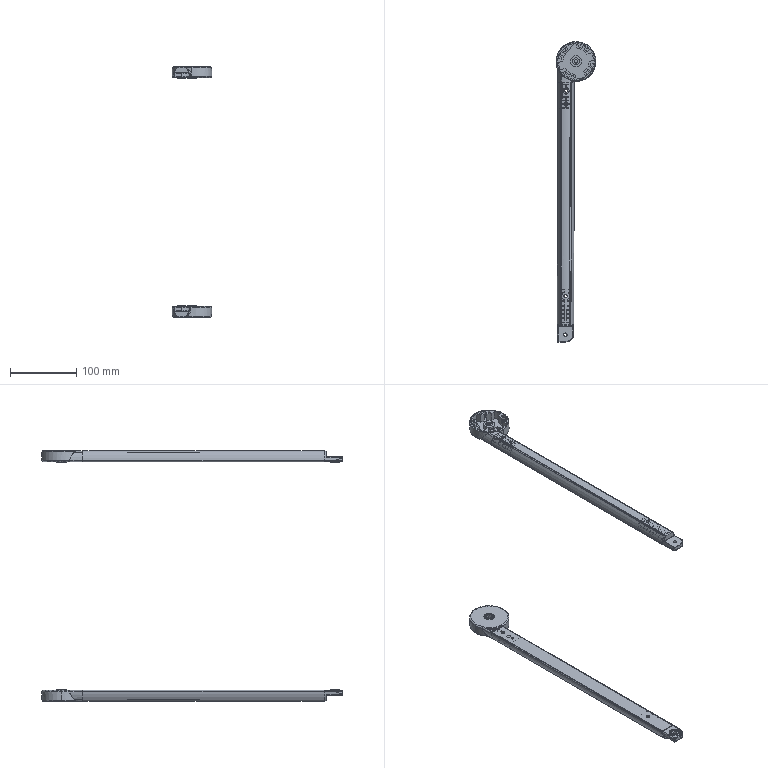Part | SolidWorks | 6 solids | 1134 faces | box 59.608 x 452.387 x 376.651 mm | volume 145181 mm3 | plane 624 | cylinder 345 | spline 153 | cone 12 | commonest cylinder face diameters 3.137 x36 53.372 x34 0.98 x23 44.411 x18 1.961 x17 5.2 x16